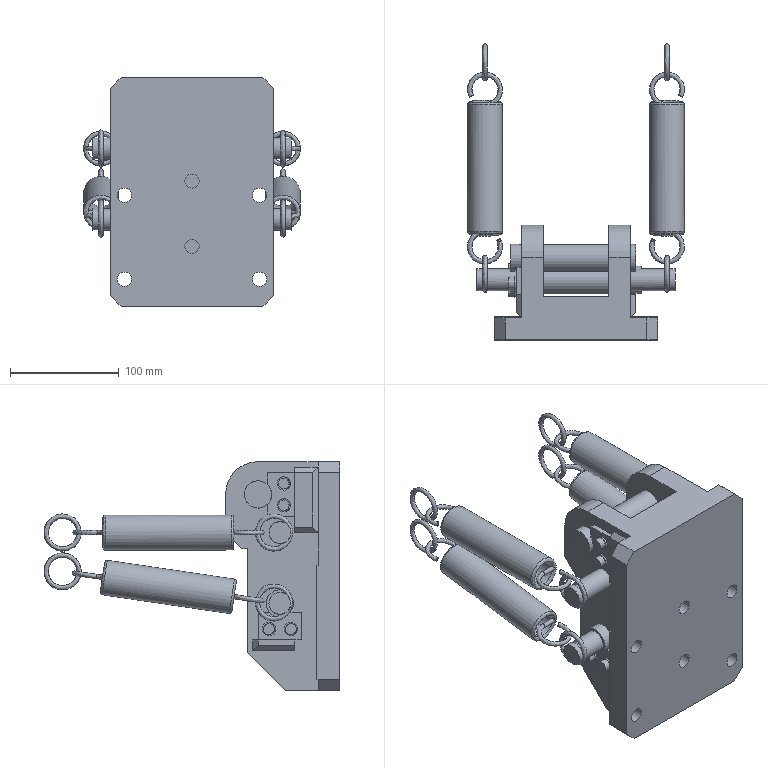Part | NX | features solid 2 | 1 solid | 248 faces | box 199 x 271.559 x 210 mm | volume 1545874 mm3 | plane 174 | cylinder 46 | spline 28 | commonest cylinder face diameters 4 x8 20 x8 13 x6 25 x6 10 x4 12.2 x4